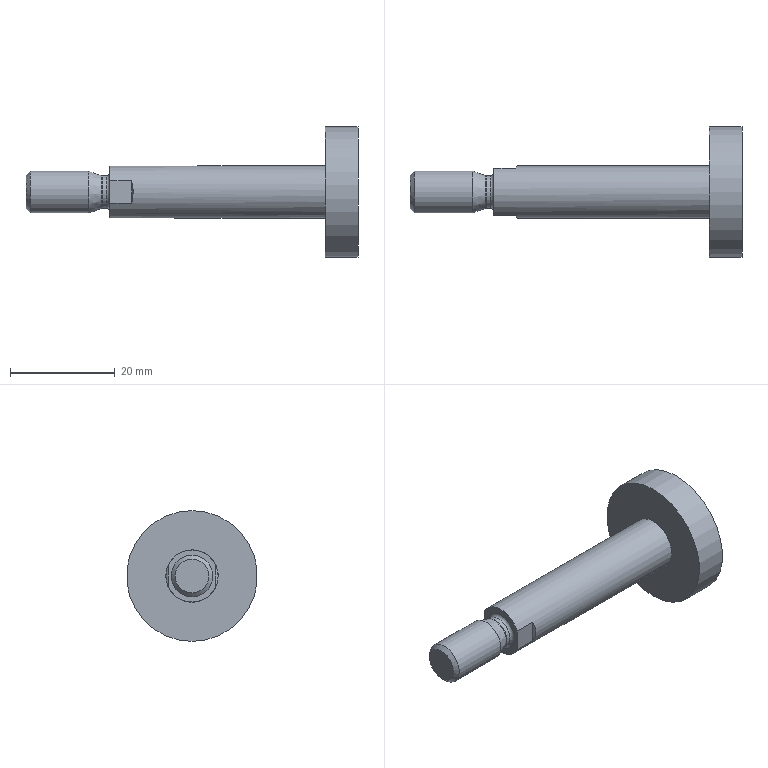Part | NX | features BREP 1 | 1 solid | 16 faces | box 63.5 x 25 x 25 mm | volume 7038 mm3 | plane 8 | cylinder 4 | cone 2 | torus 2 | commonest cylinder face diameters 6.2 x1 8 x1 10 x1 25 x1
STEP:
#1=CARTESIAN_POINT('',(35.75,0.,-5.));
#2=VERTEX_POINT('',#1);
#3=CARTESIAN_POINT('',(35.75,0.,0.));
#4=DIRECTION('',(1.,0.,0.));
#5=DIRECTION('',(0.,0.,-1.));
#6=AXIS2_PLACEMENT_3D('',#3,#4,#5);
#7=CIRCLE('',#6,5.);
#8=EDGE_CURVE('',#2,#2,#7,.T.);
#9=ORIENTED_EDGE('',*,*,#8,.F.);
#10=EDGE_LOOP('',(#9));
#11=FACE_BOUND('',#10,.T.);
#12=CARTESIAN_POINT('',(-5.5,-4.5,-2.179));
#13=VERTEX_POINT('',#12);
#14=CARTESIAN_POINT('',(-1.3,-4.5,-2.179));
#15=VERTEX_POINT('',#14);
#16=CARTESIAN_POINT('',(42.,-4.5,-2.179));
#17=DIRECTION('',(1.,0.,0.));
#18=VECTOR('',#17,1000.);
#19=LINE('',#16,#18);
#20=EDGE_CURVE('',#13,#15,#19,.T.);
#21=ORIENTED_EDGE('',*,*,#20,.F.);
#22=CARTESIAN_POINT('',(-5.5,4.5,-2.179));
#23=VERTEX_POINT('',#22);
#24=CARTESIAN_POINT('',(-5.5,0.,0.));
#25=DIRECTION('',(1.,0.,0.));
#26=DIRECTION('',(0.,0.,-1.));
#27=AXIS2_PLACEMENT_3D('',#24,#25,#26);
#28=CIRCLE('',#27,5.);
#29=EDGE_CURVE('',#13,#23,#28,.T.);
#30=ORIENTED_EDGE('',*,*,#29,.T.);
#31=CARTESIAN_POINT('',(-1.3,4.5,-2.179));
#32=VERTEX_POINT('',#31);
#33=CARTESIAN_POINT('',(42.,4.5,-2.179));
#34=DIRECTION('',(-1.,0.,0.));
#35=VECTOR('',#34,1000.);
#36=LINE('',#33,#35);
#37=EDGE_CURVE('',#32,#23,#36,.T.);
#38=ORIENTED_EDGE('',*,*,#37,.F.);
#39=CARTESIAN_POINT('',(-1.3,4.5,2.179));
#40=VERTEX_POINT('',#39);
#41=CARTESIAN_POINT('',(-1.3,4.5,2.179));
#42=CARTESIAN_POINT('',(-0.9082,5.179,0.7784));
#43=CARTESIAN_POINT('',(-0.9082,5.179,-0.7784));
#44=CARTESIAN_POINT('',(-1.3,4.5,-2.179));
#45=(BOUNDED_CURVE()B_SPLINE_CURVE(3,(#41,#42,#43,#44),.UNSPECIFIED.,.F.,.F.)B_SPLINE_CURVE_WITH_KNOTS((4,4),(0.,1.),.PIECEWISE_BEZIER_KNOTS.)CURVE()GEOMETRIC_REPRESENTATION_ITEM()RATIONAL_B_SPLINE_CURVE((1.,0.9333,0.9333,1.))REPRESENTATION_ITEM(''));
#46=EDGE_CURVE('',#40,#32,#45,.T.);
#47=ORIENTED_EDGE('',*,*,#46,.F.);
#48=CARTESIAN_POINT('',(-5.5,4.5,2.179));
#49=VERTEX_POINT('',#48);
#50=CARTESIAN_POINT('',(42.,4.5,2.179));
#51=DIRECTION('',(1.,0.,0.));
#52=VECTOR('',#51,1000.);
#53=LINE('',#50,#52);
#54=EDGE_CURVE('',#49,#40,#53,.T.);
#55=ORIENTED_EDGE('',*,*,#54,.F.);
#56=CARTESIAN_POINT('',(-5.5,-4.5,2.179));
#57=VERTEX_POINT('',#56);
#58=CARTESIAN_POINT('',(-5.5,0.,0.));
#59=DIRECTION('',(1.,0.,0.));
#60=DIRECTION('',(0.,0.,-1.));
#61=AXIS2_PLACEMENT_3D('',#58,#59,#60);
#62=CIRCLE('',#61,5.);
#63=EDGE_CURVE('',#49,#57,#62,.T.);
#64=ORIENTED_EDGE('',*,*,#63,.T.);
#65=CARTESIAN_POINT('',(-1.3,-4.5,2.179));
#66=VERTEX_POINT('',#65);
#67=CARTESIAN_POINT('',(42.,-4.5,2.179));
#68=DIRECTION('',(-1.,0.,0.));
#69=VECTOR('',#68,1000.);
#70=LINE('',#67,#69);
#71=EDGE_CURVE('',#66,#57,#70,.T.);
#72=ORIENTED_EDGE('',*,*,#71,.F.);
#73=CARTESIAN_POINT('',(-1.3,-4.5,-2.179));
#74=CARTESIAN_POINT('',(-0.9082,-5.179,-0.7784));
#75=CARTESIAN_POINT('',(-0.9082,-5.179,0.7784));
#76=CARTESIAN_POINT('',(-1.3,-4.5,2.179));
#77=(BOUNDED_CURVE()B_SPLINE_CURVE(3,(#73,#74,#75,#76),.UNSPECIFIED.,.F.,.F.)B_SPLINE_CURVE_WITH_KNOTS((4,4),(0.,1.),.PIECEWISE_BEZIER_KNOTS.)CURVE()GEOMETRIC_REPRESENTATION_ITEM()RATIONAL_B_SPLINE_CURVE((1.,0.9333,0.9333,1.))REPRESENTATION_ITEM(''));
#78=EDGE_CURVE('',#15,#66,#77,.T.);
#79=ORIENTED_EDGE('',*,*,#78,.F.);
#80=EDGE_LOOP('',(#21,#30,#38,#47,#55,#64,#72,#79));
#81=FACE_BOUND('',#80,.T.);
#82=CARTESIAN_POINT('',(42.,0.,0.));
#83=DIRECTION('',(1.,0.,0.));
#84=DIRECTION('',(0.,0.,1.));
#85=AXIS2_PLACEMENT_3D('',#82,#83,#84);
#86=CYLINDRICAL_SURFACE('',#85,5.);
#87=ADVANCED_FACE('',(#11,#81),#86,.T.);
#88=CARTESIAN_POINT('',(-5.5,4.5,0.));
#89=DIRECTION('',(0.,0.,1.));
#90=VECTOR('',#89,1000.);
#91=LINE('',#88,#90);
#92=EDGE_CURVE('',#23,#49,#91,.T.);
#93=ORIENTED_EDGE('',*,*,#92,.F.);
#94=ORIENTED_EDGE('',*,*,#29,.F.);
#95=CARTESIAN_POINT('',(-5.5,-4.5,0.));
#96=DIRECTION('',(0.,0.,-1.));
#97=VECTOR('',#96,1000.);
#98=LINE('',#95,#97);
#99=EDGE_CURVE('',#57,#13,#98,.T.);
#100=ORIENTED_EDGE('',*,*,#99,.F.);
#101=ORIENTED_EDGE('',*,*,#63,.F.);
#102=EDGE_LOOP('',(#93,#94,#100,#101));
#103=FACE_BOUND('',#102,.T.);
#104=CARTESIAN_POINT('',(-5.5,0.,-3.7));
#105=VERTEX_POINT('',#104);
#106=CARTESIAN_POINT('',(-5.5,0.,0.));
#107=DIRECTION('',(1.,0.,0.));
#108=DIRECTION('',(0.,0.,-1.));
#109=AXIS2_PLACEMENT_3D('',#106,#107,#108);
#110=CIRCLE('',#109,3.7);
#111=EDGE_CURVE('',#105,#105,#110,.T.);
#112=ORIENTED_EDGE('',*,*,#111,.T.);
#113=EDGE_LOOP('',(#112));
#114=FACE_BOUND('',#113,.T.);
#115=CARTESIAN_POINT('',(-5.5,0.,0.));
#116=DIRECTION('',(1.,0.,0.));
#117=DIRECTION('',(0.,0.,1.));
#118=AXIS2_PLACEMENT_3D('',#115,#116,#117);
#119=PLANE('',#118);
#120=ADVANCED_FACE('',(#103,#114),#119,.F.);
#121=CARTESIAN_POINT('',(35.75,0.,-12.5));
#122=VERTEX_POINT('',#121);
#123=CARTESIAN_POINT('',(35.75,0.,0.));
#124=DIRECTION('',(1.,0.,0.));
#125=DIRECTION('',(0.,0.,-1.));
#126=AXIS2_PLACEMENT_3D('',#123,#124,#125);
#127=CIRCLE('',#126,12.5);
#128=EDGE_CURVE('',#122,#122,#127,.T.);
#129=ORIENTED_EDGE('',*,*,#128,.F.);
#130=EDGE_LOOP('',(#129));
#131=FACE_BOUND('',#130,.T.);
#132=ORIENTED_EDGE('',*,*,#8,.T.);
#133=EDGE_LOOP('',(#132));
#134=FACE_BOUND('',#133,.T.);
#135=CARTESIAN_POINT('',(35.75,0.,0.));
#136=DIRECTION('',(1.,0.,0.));
#137=DIRECTION('',(0.,0.,1.));
#138=AXIS2_PLACEMENT_3D('',#135,#136,#137);
#139=PLANE('',#138);
#140=ADVANCED_FACE('',(#131,#134),#139,.F.);
#141=CARTESIAN_POINT('',(42.,0.,-12.5));
#142=VERTEX_POINT('',#141);
#143=CARTESIAN_POINT('',(42.,0.,0.));
#144=DIRECTION('',(1.,0.,0.));
#145=DIRECTION('',(0.,0.,-1.));
#146=AXIS2_PLACEMENT_3D('',#143,#144,#145);
#147=CIRCLE('',#146,12.5);
#148=EDGE_CURVE('',#142,#142,#147,.T.);
#149=ORIENTED_EDGE('',*,*,#148,.F.);
#150=EDGE_LOOP('',(#149));
#151=FACE_BOUND('',#150,.T.);
#152=ORIENTED_EDGE('',*,*,#128,.T.);
#153=EDGE_LOOP('',(#152));
#154=FACE_BOUND('',#153,.T.);
#155=CARTESIAN_POINT('',(42.,0.,0.));
#156=DIRECTION('',(1.,0.,0.));
#157=DIRECTION('',(0.,0.,1.));
#158=AXIS2_PLACEMENT_3D('',#155,#156,#157);
#159=CYLINDRICAL_SURFACE('',#158,12.5);
#160=ADVANCED_FACE('',(#151,#154),#159,.T.);
#161=ORIENTED_EDGE('',*,*,#148,.T.);
#162=EDGE_LOOP('',(#161));
#163=FACE_BOUND('',#162,.T.);
#164=CARTESIAN_POINT('',(42.,5.,0.));
#165=DIRECTION('',(-1.,0.,0.));
#166=DIRECTION('',(0.,0.,-1.));
#167=AXIS2_PLACEMENT_3D('',#164,#165,#166);
#168=PLANE('',#167);
#169=ADVANCED_FACE('',(#163),#168,.F.);
#170=CARTESIAN_POINT('',(-21.5,0.,-3.233));
#171=VERTEX_POINT('',#170);
#172=CARTESIAN_POINT('',(-21.5,0.,0.));
#173=DIRECTION('',(1.,0.,0.));
#174=DIRECTION('',(0.,0.,-1.));
#175=AXIS2_PLACEMENT_3D('',#172,#173,#174);
#176=CIRCLE('',#175,3.233);
#177=EDGE_CURVE('',#171,#171,#176,.T.);
#178=ORIENTED_EDGE('',*,*,#177,.F.);
#179=EDGE_LOOP('',(#178));
#180=FACE_BOUND('',#179,.T.);
#181=CARTESIAN_POINT('',(-21.5,0.,0.));
#182=DIRECTION('',(1.,0.,0.));
#183=DIRECTION('',(0.,0.,1.));
#184=AXIS2_PLACEMENT_3D('',#181,#182,#183);
#185=PLANE('',#184);
#186=ADVANCED_FACE('',(#180),#185,.F.);
#187=CARTESIAN_POINT('',(-20.733,0.,-4.));
#188=VERTEX_POINT('',#187);
#189=CARTESIAN_POINT('',(-20.733,0.,0.));
#190=DIRECTION('',(1.,0.,0.));
#191=DIRECTION('',(0.,0.,-1.));
#192=AXIS2_PLACEMENT_3D('',#189,#190,#191);
#193=CIRCLE('',#192,4.);
#194=EDGE_CURVE('',#188,#188,#193,.T.);
#195=ORIENTED_EDGE('',*,*,#194,.F.);
#196=EDGE_LOOP('',(#195));
#197=FACE_BOUND('',#196,.T.);
#198=ORIENTED_EDGE('',*,*,#177,.T.);
#199=EDGE_LOOP('',(#198));
#200=FACE_BOUND('',#199,.T.);
#201=CARTESIAN_POINT('',(-21.5,0.,0.));
#202=DIRECTION('',(1.,0.,0.));
#203=DIRECTION('',(0.,0.,1.));
#204=AXIS2_PLACEMENT_3D('',#201,#202,#203);
#205=CONICAL_SURFACE('',#204,3.233,0.7854);
#206=ADVANCED_FACE('',(#197,#200),#205,.T.);
#207=CARTESIAN_POINT('',(-9.473,0.,-4.));
#208=VERTEX_POINT('',#207);
#209=CARTESIAN_POINT('',(-9.473,0.,0.));
#210=DIRECTION('',(1.,0.,0.));
#211=DIRECTION('',(0.,0.,-1.));
#212=AXIS2_PLACEMENT_3D('',#209,#210,#211);
#213=CIRCLE('',#212,4.);
#214=EDGE_CURVE('',#208,#208,#213,.T.);
#215=ORIENTED_EDGE('',*,*,#214,.F.);
#216=EDGE_LOOP('',(#215));
#217=FACE_BOUND('',#216,.T.);
#218=ORIENTED_EDGE('',*,*,#194,.T.);
#219=EDGE_LOOP('',(#218));
#220=FACE_BOUND('',#219,.T.);
#221=CARTESIAN_POINT('',(-4.5,0.,0.));
#222=DIRECTION('',(1.,0.,0.));
#223=DIRECTION('',(0.,0.,1.));
#224=AXIS2_PLACEMENT_3D('',#221,#222,#223);
#225=CYLINDRICAL_SURFACE('',#224,4.);
#226=ADVANCED_FACE('',(#217,#220),#225,.T.);
#227=CARTESIAN_POINT('',(-7.099,0.,-3.136));
#228=VERTEX_POINT('',#227);
#229=CARTESIAN_POINT('',(-7.099,0.,0.));
#230=DIRECTION('',(1.,0.,0.));
#231=DIRECTION('',(0.,0.,-1.));
#232=AXIS2_PLACEMENT_3D('',#229,#230,#231);
#233=CIRCLE('',#232,3.136);
#234=EDGE_CURVE('',#228,#228,#233,.T.);
#235=ORIENTED_EDGE('',*,*,#234,.F.);
#236=EDGE_LOOP('',(#235));
#237=FACE_BOUND('',#236,.T.);
#238=ORIENTED_EDGE('',*,*,#214,.T.);
#239=EDGE_LOOP('',(#238));
#240=FACE_BOUND('',#239,.T.);
#241=CARTESIAN_POINT('',(-9.473,0.,0.));
#242=DIRECTION('',(-1.,0.,0.));
#243=DIRECTION('',(0.,0.,-1.));
#244=AXIS2_PLACEMENT_3D('',#241,#242,#243);
#245=CONICAL_SURFACE('',#244,4.,0.3491);
#246=ADVANCED_FACE('',(#237,#240),#245,.T.);
#247=CARTESIAN_POINT('',(-6.894,0.,-3.1));
#248=VERTEX_POINT('',#247);
#249=CARTESIAN_POINT('',(-6.894,0.,0.));
#250=DIRECTION('',(1.,0.,0.));
#251=DIRECTION('',(0.,0.,-1.));
#252=AXIS2_PLACEMENT_3D('',#249,#250,#251);
#253=CIRCLE('',#252,3.1);
#254=EDGE_CURVE('',#248,#248,#253,.T.);
#255=ORIENTED_EDGE('',*,*,#254,.F.);
#256=EDGE_LOOP('',(#255));
#257=FACE_BOUND('',#256,.T.);
#258=ORIENTED_EDGE('',*,*,#234,.T.);
#259=EDGE_LOOP('',(#258));
#260=FACE_BOUND('',#259,.T.);
#261=CARTESIAN_POINT('',(-6.894,0.,0.));
#262=DIRECTION('',(1.,0.,0.));
#263=DIRECTION('',(0.,0.,1.));
#264=AXIS2_PLACEMENT_3D('',#261,#262,#263);
#265=TOROIDAL_SURFACE('',#264,3.7,0.6);
#266=ADVANCED_FACE('',(#257,#260),#265,.F.);
#267=CARTESIAN_POINT('',(-6.1,0.,-3.1));
#268=VERTEX_POINT('',#267);
#269=CARTESIAN_POINT('',(-6.1,0.,0.));
#270=DIRECTION('',(1.,0.,0.));
#271=DIRECTION('',(0.,0.,-1.));
#272=AXIS2_PLACEMENT_3D('',#269,#270,#271);
#273=CIRCLE('',#272,3.1);
#274=EDGE_CURVE('',#268,#268,#273,.T.);
#275=ORIENTED_EDGE('',*,*,#274,.F.);
#276=EDGE_LOOP('',(#275));
#277=FACE_BOUND('',#276,.T.);
#278=ORIENTED_EDGE('',*,*,#254,.T.);
#279=EDGE_LOOP('',(#278));
#280=FACE_BOUND('',#279,.T.);
#281=CARTESIAN_POINT('',(-4.5,0.,0.));
#282=DIRECTION('',(1.,0.,0.));
#283=DIRECTION('',(0.,0.,1.));
#284=AXIS2_PLACEMENT_3D('',#281,#282,#283);
#285=CYLINDRICAL_SURFACE('',#284,3.1);
#286=ADVANCED_FACE('',(#277,#280),#285,.T.);
#287=ORIENTED_EDGE('',*,*,#111,.F.);
#288=EDGE_LOOP('',(#287));
#289=FACE_BOUND('',#288,.T.);
#290=ORIENTED_EDGE('',*,*,#274,.T.);
#291=EDGE_LOOP('',(#290));
#292=FACE_BOUND('',#291,.T.);
#293=CARTESIAN_POINT('',(-6.1,0.,0.));
#294=DIRECTION('',(1.,0.,0.));
#295=DIRECTION('',(0.,0.,1.));
#296=AXIS2_PLACEMENT_3D('',#293,#294,#295);
#297=TOROIDAL_SURFACE('',#296,3.7,0.6);
#298=ADVANCED_FACE('',(#289,#292),#297,.F.);
#299=ORIENTED_EDGE('',*,*,#54,.T.);
#300=CARTESIAN_POINT('',(-1.3,4.5,10.));
#301=DIRECTION('',(0.,0.,-1.));
#302=VECTOR('',#301,1000.);
#303=LINE('',#300,#302);
#304=EDGE_CURVE('',#40,#32,#303,.T.);
#305=ORIENTED_EDGE('',*,*,#304,.T.);
#306=ORIENTED_EDGE('',*,*,#37,.T.);
#307=ORIENTED_EDGE('',*,*,#92,.T.);
#308=EDGE_LOOP('',(#299,#305,#306,#307));
#309=FACE_BOUND('',#308,.T.);
#310=CARTESIAN_POINT('',(-5.5,4.5,10.));
#311=DIRECTION('',(0.,1.,0.));
#312=DIRECTION('',(0.,0.,-1.));
#313=AXIS2_PLACEMENT_3D('',#310,#311,#312);
#314=PLANE('',#313);
#315=ADVANCED_FACE('',(#309),#314,.T.);
#316=ORIENTED_EDGE('',*,*,#46,.T.);
#317=ORIENTED_EDGE('',*,*,#304,.F.);
#318=EDGE_LOOP('',(#316,#317));
#319=FACE_BOUND('',#318,.T.);
#320=CARTESIAN_POINT('',(-1.3,4.5,10.));
#321=DIRECTION('',(-0.866,0.5,0.));
#322=DIRECTION('',(0.5,0.866,0.));
#323=AXIS2_PLACEMENT_3D('',#320,#321,#322);
#324=PLANE('',#323);
#325=ADVANCED_FACE('',(#319),#324,.T.);
#326=ORIENTED_EDGE('',*,*,#78,.T.);
#327=CARTESIAN_POINT('',(-1.3,-4.5,10.));
#328=DIRECTION('',(0.,0.,-1.));
#329=VECTOR('',#328,1000.);
#330=LINE('',#327,#329);
#331=EDGE_CURVE('',#66,#15,#330,.T.);
#332=ORIENTED_EDGE('',*,*,#331,.T.);
#333=EDGE_LOOP('',(#326,#332));
#334=FACE_BOUND('',#333,.T.);
#335=CARTESIAN_POINT('',(4.474,-14.5,10.));
#336=DIRECTION('',(-0.866,-0.5,0.));
#337=DIRECTION('',(-0.5,0.866,0.));
#338=AXIS2_PLACEMENT_3D('',#335,#336,#337);
#339=PLANE('',#338);
#340=ADVANCED_FACE('',(#334),#339,.T.);
#341=ORIENTED_EDGE('',*,*,#20,.T.);
#342=ORIENTED_EDGE('',*,*,#331,.F.);
#343=ORIENTED_EDGE('',*,*,#71,.T.);
#344=ORIENTED_EDGE('',*,*,#99,.T.);
#345=EDGE_LOOP('',(#341,#342,#343,#344));
#346=FACE_BOUND('',#345,.T.);
#347=CARTESIAN_POINT('',(-1.3,-4.5,10.));
#348=DIRECTION('',(0.,-1.,0.));
#349=DIRECTION('',(0.,0.,1.));
#350=AXIS2_PLACEMENT_3D('',#347,#348,#349);
#351=PLANE('',#350);
#352=ADVANCED_FACE('',(#346),#351,.T.);
#353=CLOSED_SHELL('',(#87,#120,#140,#160,#169,#186,#206,#226,#246,#266,#286,#298,#315,#325,#340,#352));
#354=MANIFOLD_SOLID_BREP('',#353);
#355=(LENGTH_UNIT()NAMED_UNIT(*)SI_UNIT(.MILLI.,.METRE.));
#356=UNCERTAINTY_MEASURE_WITH_UNIT(LENGTH_MEASURE(0.00001),#355,'','');
#357=(NAMED_UNIT(*)PLANE_ANGLE_UNIT()SI_UNIT($,.RADIAN.));
#358=(NAMED_UNIT(*)SI_UNIT($,.STERADIAN.)SOLID_ANGLE_UNIT());
#359=(GEOMETRIC_REPRESENTATION_CONTEXT(3)GLOBAL_UNCERTAINTY_ASSIGNED_CONTEXT((#356))GLOBAL_UNIT_ASSIGNED_CONTEXT((#355,#357,#358))REPRESENTATION_CONTEXT('',''));
#360=ADVANCED_BREP_SHAPE_REPRESENTATION('',(#354),#359);